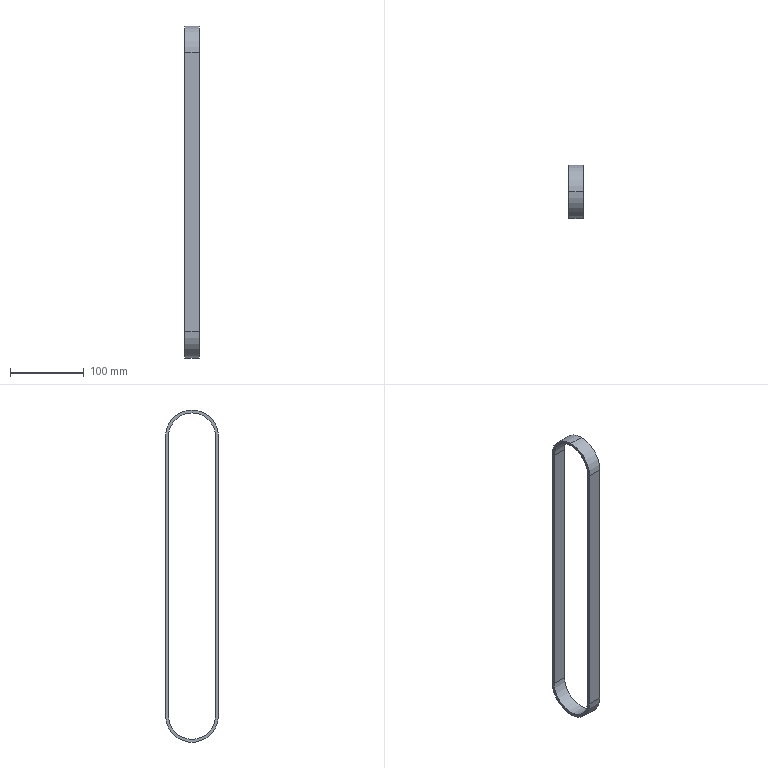Part | STEP file | PN_0034 (conveyor belt) | 1 solid | 12 faces | box 20 x 72 x 452 mm | volume 77890 mm3 | cylinder 6 | plane 6 | commonest cylinder face diameters 64 x3 72 x3
STEP:
#1=CARTESIAN_POINT('',(0.,0.,0.));
#2=DIRECTION('',(0.,0.,1.));
#3=DIRECTION('',(1.,0.,0.));
#4=AXIS2_PLACEMENT_3D('',#1,#2,#3);
#5=CARTESIAN_POINT('',(10.,32.,0.));
#6=VERTEX_POINT('',#5);
#7=CARTESIAN_POINT('',(-10.,32.,0.));
#8=VERTEX_POINT('',#7);
#9=CARTESIAN_POINT('',(10.,32.,0.));
#10=DIRECTION('',(-1.,0.,0.));
#11=VECTOR('',#10,1.);
#12=LINE('',#9,#11);
#13=CARTESIAN_POINT('',(10.,0.,0.));
#14=DIRECTION('',(-1.,0.,0.));
#15=DIRECTION('',(0.,0.,1.));
#16=AXIS2_PLACEMENT_3D('',#13,#14,#15);
#17=CYLINDRICAL_SURFACE('',#16,32.);
#18=CARTESIAN_POINT('',(1.571,0.));
#19=DIRECTION('',(0.,1.));
#20=VECTOR('',#19,1.);
#21=LINE('',#18,#20);
#22=(GEOMETRIC_REPRESENTATION_CONTEXT(2)PARAMETRIC_REPRESENTATION_CONTEXT()REPRESENTATION_CONTEXT('',''));
#23=DEFINITIONAL_REPRESENTATION('',(#21),#22);
#24=PCURVE('',#17,#23);
#25=CARTESIAN_POINT('',(10.,32.,0.));
#26=DIRECTION('',(0.,-1.,0.));
#27=DIRECTION('',(0.,0.,-1.));
#28=AXIS2_PLACEMENT_3D('',#25,#26,#27);
#29=PLANE('',#28);
#30=CARTESIAN_POINT('',(0.,0.));
#31=DIRECTION('',(0.,-1.));
#32=VECTOR('',#31,1.);
#33=LINE('',#30,#32);
#34=(GEOMETRIC_REPRESENTATION_CONTEXT(2)PARAMETRIC_REPRESENTATION_CONTEXT()REPRESENTATION_CONTEXT('',''));
#35=DEFINITIONAL_REPRESENTATION('',(#33),#34);
#36=PCURVE('',#29,#35);
#37=SURFACE_CURVE('',#12,(#24,#36),.PCURVE_S1.);
#38=EDGE_CURVE('',#6,#8,#37,.T.);
#39=ORIENTED_EDGE('',*,*,#38,.T.);
#40=CARTESIAN_POINT('',(-10.,0.,32.));
#41=VERTEX_POINT('',#40);
#42=CARTESIAN_POINT('',(-10.,0.,0.));
#43=DIRECTION('',(1.,0.,0.));
#44=DIRECTION('',(0.,0.,-1.));
#45=AXIS2_PLACEMENT_3D('',#42,#43,#44);
#46=CIRCLE('',#45,32.);
#47=CARTESIAN_POINT('',(3.142,20.));
#48=DIRECTION('',(-1.,0.));
#49=VECTOR('',#48,1.);
#50=LINE('',#47,#49);
#51=(GEOMETRIC_REPRESENTATION_CONTEXT(2)PARAMETRIC_REPRESENTATION_CONTEXT()REPRESENTATION_CONTEXT('',''));
#52=DEFINITIONAL_REPRESENTATION('',(#50),#51);
#53=PCURVE('',#17,#52);
#54=CARTESIAN_POINT('',(-10.,0.,0.));
#55=DIRECTION('',(1.,0.,0.));
#56=DIRECTION('',(0.,0.,-1.));
#57=AXIS2_PLACEMENT_3D('',#54,#55,#56);
#58=PLANE('',#57);
#59=CARTESIAN_POINT('',(0.,0.));
#60=DIRECTION('',(1.,0.));
#61=AXIS2_PLACEMENT_2D('',#59,#60);
#62=CIRCLE('',#61,32.);
#63=(GEOMETRIC_REPRESENTATION_CONTEXT(2)PARAMETRIC_REPRESENTATION_CONTEXT()REPRESENTATION_CONTEXT('',''));
#64=DEFINITIONAL_REPRESENTATION('',(#62),#63);
#65=PCURVE('',#58,#64);
#66=SURFACE_CURVE('',#46,(#53,#65),.PCURVE_S1.);
#67=EDGE_CURVE('',#8,#41,#66,.T.);
#68=ORIENTED_EDGE('',*,*,#67,.T.);
#69=CARTESIAN_POINT('',(10.,0.,32.));
#70=VERTEX_POINT('',#69);
#71=CARTESIAN_POINT('',(10.,0.,32.));
#72=DIRECTION('',(-1.,0.,0.));
#73=VECTOR('',#72,1.);
#74=LINE('',#71,#73);
#75=CARTESIAN_POINT('',(0.,0.));
#76=DIRECTION('',(0.,1.));
#77=VECTOR('',#76,1.);
#78=LINE('',#75,#77);
#79=(GEOMETRIC_REPRESENTATION_CONTEXT(2)PARAMETRIC_REPRESENTATION_CONTEXT()REPRESENTATION_CONTEXT('',''));
#80=DEFINITIONAL_REPRESENTATION('',(#78),#79);
#81=PCURVE('',#17,#80);
#82=CARTESIAN_POINT('',(10.,0.,0.));
#83=DIRECTION('',(-1.,0.,0.));
#84=DIRECTION('',(0.,0.,1.));
#85=AXIS2_PLACEMENT_3D('',#82,#83,#84);
#86=CYLINDRICAL_SURFACE('',#85,32.);
#87=CARTESIAN_POINT('',(6.283,0.));
#88=DIRECTION('',(0.,1.));
#89=VECTOR('',#88,1.);
#90=LINE('',#87,#89);
#91=(GEOMETRIC_REPRESENTATION_CONTEXT(2)PARAMETRIC_REPRESENTATION_CONTEXT()REPRESENTATION_CONTEXT('',''));
#92=DEFINITIONAL_REPRESENTATION('',(#90),#91);
#93=PCURVE('',#86,#92);
#94=SURFACE_CURVE('',#74,(#81,#93),.PCURVE_S1.);
#95=EDGE_CURVE('',#70,#41,#94,.T.);
#96=ORIENTED_EDGE('',*,*,#95,.F.);
#97=CARTESIAN_POINT('',(10.,0.,0.));
#98=DIRECTION('',(1.,0.,0.));
#99=DIRECTION('',(0.,0.,-1.));
#100=AXIS2_PLACEMENT_3D('',#97,#98,#99);
#101=CIRCLE('',#100,32.);
#102=CARTESIAN_POINT('',(3.142,0.));
#103=DIRECTION('',(-1.,0.));
#104=VECTOR('',#103,1.);
#105=LINE('',#102,#104);
#106=(GEOMETRIC_REPRESENTATION_CONTEXT(2)PARAMETRIC_REPRESENTATION_CONTEXT()REPRESENTATION_CONTEXT('',''));
#107=DEFINITIONAL_REPRESENTATION('',(#105),#106);
#108=PCURVE('',#17,#107);
#109=CARTESIAN_POINT('',(10.,0.,0.));
#110=DIRECTION('',(1.,0.,0.));
#111=DIRECTION('',(0.,0.,-1.));
#112=AXIS2_PLACEMENT_3D('',#109,#110,#111);
#113=PLANE('',#112);
#114=CARTESIAN_POINT('',(0.,0.));
#115=DIRECTION('',(1.,0.));
#116=AXIS2_PLACEMENT_2D('',#114,#115);
#117=CIRCLE('',#116,32.);
#118=(GEOMETRIC_REPRESENTATION_CONTEXT(2)PARAMETRIC_REPRESENTATION_CONTEXT()REPRESENTATION_CONTEXT('',''));
#119=DEFINITIONAL_REPRESENTATION('',(#117),#118);
#120=PCURVE('',#113,#119);
#121=SURFACE_CURVE('',#101,(#108,#120),.PCURVE_S1.);
#122=EDGE_CURVE('',#6,#70,#121,.T.);
#123=ORIENTED_EDGE('',*,*,#122,.F.);
#124=EDGE_LOOP('',(#39,#68,#96,#123));
#125=FACE_BOUND('',#124,.F.);
#126=ADVANCED_FACE('',(#125),#17,.F.);
#127=CARTESIAN_POINT('',(10.,0.,36.));
#128=VERTEX_POINT('',#127);
#129=CARTESIAN_POINT('',(10.,-36.,0.));
#130=VERTEX_POINT('',#129);
#131=CARTESIAN_POINT('',(10.,0.,0.));
#132=DIRECTION('',(1.,0.,0.));
#133=DIRECTION('',(0.,0.,-1.));
#134=AXIS2_PLACEMENT_3D('',#131,#132,#133);
#135=CIRCLE('',#134,36.);
#136=CARTESIAN_POINT('',(10.,0.,0.));
#137=DIRECTION('',(-1.,0.,0.));
#138=DIRECTION('',(0.,0.,1.));
#139=AXIS2_PLACEMENT_3D('',#136,#137,#138);
#140=CYLINDRICAL_SURFACE('',#139,36.);
#141=CARTESIAN_POINT('',(9.425,0.));
#142=DIRECTION('',(-1.,0.));
#143=VECTOR('',#142,1.);
#144=LINE('',#141,#143);
#145=(GEOMETRIC_REPRESENTATION_CONTEXT(2)PARAMETRIC_REPRESENTATION_CONTEXT()REPRESENTATION_CONTEXT('',''));
#146=DEFINITIONAL_REPRESENTATION('',(#144),#145);
#147=PCURVE('',#140,#146);
#148=CARTESIAN_POINT('',(0.,0.));
#149=DIRECTION('',(1.,0.));
#150=AXIS2_PLACEMENT_2D('',#148,#149);
#151=CIRCLE('',#150,36.);
#152=(GEOMETRIC_REPRESENTATION_CONTEXT(2)PARAMETRIC_REPRESENTATION_CONTEXT()REPRESENTATION_CONTEXT('',''));
#153=DEFINITIONAL_REPRESENTATION('',(#151),#152);
#154=PCURVE('',#113,#153);
#155=SURFACE_CURVE('',#135,(#147,#154),.PCURVE_S1.);
#156=EDGE_CURVE('',#128,#130,#155,.T.);
#157=ORIENTED_EDGE('',*,*,#156,.F.);
#158=CARTESIAN_POINT('',(-10.,0.,36.));
#159=VERTEX_POINT('',#158);
#160=CARTESIAN_POINT('',(10.,0.,36.));
#161=DIRECTION('',(-1.,0.,0.));
#162=VECTOR('',#161,1.);
#163=LINE('',#160,#162);
#164=CARTESIAN_POINT('',(6.283,0.));
#165=DIRECTION('',(0.,1.));
#166=VECTOR('',#165,1.);
#167=LINE('',#164,#166);
#168=(GEOMETRIC_REPRESENTATION_CONTEXT(2)PARAMETRIC_REPRESENTATION_CONTEXT()REPRESENTATION_CONTEXT('',''));
#169=DEFINITIONAL_REPRESENTATION('',(#167),#168);
#170=PCURVE('',#140,#169);
#171=CARTESIAN_POINT('',(10.,0.,0.));
#172=DIRECTION('',(-1.,0.,0.));
#173=DIRECTION('',(0.,0.,1.));
#174=AXIS2_PLACEMENT_3D('',#171,#172,#173);
#175=CYLINDRICAL_SURFACE('',#174,36.);
#176=CARTESIAN_POINT('',(0.,0.));
#177=DIRECTION('',(0.,1.));
#178=VECTOR('',#177,1.);
#179=LINE('',#176,#178);
#180=(GEOMETRIC_REPRESENTATION_CONTEXT(2)PARAMETRIC_REPRESENTATION_CONTEXT()REPRESENTATION_CONTEXT('',''));
#181=DEFINITIONAL_REPRESENTATION('',(#179),#180);
#182=PCURVE('',#175,#181);
#183=SURFACE_CURVE('',#163,(#170,#182),.PCURVE_S1.);
#184=EDGE_CURVE('',#128,#159,#183,.T.);
#185=ORIENTED_EDGE('',*,*,#184,.T.);
#186=CARTESIAN_POINT('',(-10.,-36.,0.));
#187=VERTEX_POINT('',#186);
#188=CARTESIAN_POINT('',(-10.,0.,0.));
#189=DIRECTION('',(1.,0.,0.));
#190=DIRECTION('',(0.,0.,-1.));
#191=AXIS2_PLACEMENT_3D('',#188,#189,#190);
#192=CIRCLE('',#191,36.);
#193=CARTESIAN_POINT('',(9.425,20.));
#194=DIRECTION('',(-1.,0.));
#195=VECTOR('',#194,1.);
#196=LINE('',#193,#195);
#197=(GEOMETRIC_REPRESENTATION_CONTEXT(2)PARAMETRIC_REPRESENTATION_CONTEXT()REPRESENTATION_CONTEXT('',''));
#198=DEFINITIONAL_REPRESENTATION('',(#196),#197);
#199=PCURVE('',#140,#198);
#200=CARTESIAN_POINT('',(0.,0.));
#201=DIRECTION('',(1.,0.));
#202=AXIS2_PLACEMENT_2D('',#200,#201);
#203=CIRCLE('',#202,36.);
#204=(GEOMETRIC_REPRESENTATION_CONTEXT(2)PARAMETRIC_REPRESENTATION_CONTEXT()REPRESENTATION_CONTEXT('',''));
#205=DEFINITIONAL_REPRESENTATION('',(#203),#204);
#206=PCURVE('',#58,#205);
#207=SURFACE_CURVE('',#192,(#199,#206),.PCURVE_S1.);
#208=EDGE_CURVE('',#159,#187,#207,.T.);
#209=ORIENTED_EDGE('',*,*,#208,.T.);
#210=CARTESIAN_POINT('',(10.,-36.,0.));
#211=DIRECTION('',(-1.,0.,0.));
#212=VECTOR('',#211,1.);
#213=LINE('',#210,#212);
#214=CARTESIAN_POINT('',(4.712,0.));
#215=DIRECTION('',(0.,1.));
#216=VECTOR('',#215,1.);
#217=LINE('',#214,#216);
#218=(GEOMETRIC_REPRESENTATION_CONTEXT(2)PARAMETRIC_REPRESENTATION_CONTEXT()REPRESENTATION_CONTEXT('',''));
#219=DEFINITIONAL_REPRESENTATION('',(#217),#218);
#220=PCURVE('',#140,#219);
#221=CARTESIAN_POINT('',(10.,-36.,0.));
#222=DIRECTION('',(0.,1.,0.));
#223=DIRECTION('',(0.,0.,1.));
#224=AXIS2_PLACEMENT_3D('',#221,#222,#223);
#225=PLANE('',#224);
#226=CARTESIAN_POINT('',(0.,0.));
#227=DIRECTION('',(0.,-1.));
#228=VECTOR('',#227,1.);
#229=LINE('',#226,#228);
#230=(GEOMETRIC_REPRESENTATION_CONTEXT(2)PARAMETRIC_REPRESENTATION_CONTEXT()REPRESENTATION_CONTEXT('',''));
#231=DEFINITIONAL_REPRESENTATION('',(#229),#230);
#232=PCURVE('',#225,#231);
#233=SURFACE_CURVE('',#213,(#220,#232),.PCURVE_S1.);
#234=EDGE_CURVE('',#130,#187,#233,.T.);
#235=ORIENTED_EDGE('',*,*,#234,.F.);
#236=EDGE_LOOP('',(#157,#185,#209,#235));
#237=FACE_BOUND('',#236,.T.);
#238=ADVANCED_FACE('',(#237),#140,.T.);
#239=CARTESIAN_POINT('',(10.,36.,0.));
#240=VERTEX_POINT('',#239);
#241=CARTESIAN_POINT('',(10.,0.,0.));
#242=DIRECTION('',(1.,0.,0.));
#243=DIRECTION('',(0.,0.,-1.));
#244=AXIS2_PLACEMENT_3D('',#241,#242,#243);
#245=CIRCLE('',#244,36.);
#246=CARTESIAN_POINT('',(0.,0.));
#247=DIRECTION('',(1.,0.));
#248=AXIS2_PLACEMENT_2D('',#246,#247);
#249=CIRCLE('',#248,36.);
#250=(GEOMETRIC_REPRESENTATION_CONTEXT(2)PARAMETRIC_REPRESENTATION_CONTEXT()REPRESENTATION_CONTEXT('',''));
#251=DEFINITIONAL_REPRESENTATION('',(#249),#250);
#252=PCURVE('',#113,#251);
#253=CARTESIAN_POINT('',(3.142,0.));
#254=DIRECTION('',(-1.,0.));
#255=VECTOR('',#254,1.);
#256=LINE('',#253,#255);
#257=(GEOMETRIC_REPRESENTATION_CONTEXT(2)PARAMETRIC_REPRESENTATION_CONTEXT()REPRESENTATION_CONTEXT('',''));
#258=DEFINITIONAL_REPRESENTATION('',(#256),#257);
#259=PCURVE('',#175,#258);
#260=SURFACE_CURVE('',#245,(#252,#259),.PCURVE_S1.);
#261=EDGE_CURVE('',#240,#128,#260,.T.);
#262=ORIENTED_EDGE('',*,*,#261,.T.);
#263=ORIENTED_EDGE('',*,*,#156,.T.);
#264=CARTESIAN_POINT('',(10.,-36.,-380.));
#265=VERTEX_POINT('',#264);
#266=CARTESIAN_POINT('',(10.,-36.,0.));
#267=DIRECTION('',(0.,0.,-1.));
#268=VECTOR('',#267,1.);
#269=LINE('',#266,#268);
#270=CARTESIAN_POINT('',(0.,-36.));
#271=DIRECTION('',(1.,0.));
#272=VECTOR('',#271,1.);
#273=LINE('',#270,#272);
#274=(GEOMETRIC_REPRESENTATION_CONTEXT(2)PARAMETRIC_REPRESENTATION_CONTEXT()REPRESENTATION_CONTEXT('',''));
#275=DEFINITIONAL_REPRESENTATION('',(#273),#274);
#276=PCURVE('',#113,#275);
#277=CARTESIAN_POINT('',(0.,0.));
#278=DIRECTION('',(-1.,0.));
#279=VECTOR('',#278,1.);
#280=LINE('',#277,#279);
#281=(GEOMETRIC_REPRESENTATION_CONTEXT(2)PARAMETRIC_REPRESENTATION_CONTEXT()REPRESENTATION_CONTEXT('',''));
#282=DEFINITIONAL_REPRESENTATION('',(#280),#281);
#283=PCURVE('',#225,#282);
#284=SURFACE_CURVE('',#269,(#276,#283),.PCURVE_S1.);
#285=EDGE_CURVE('',#130,#265,#284,.T.);
#286=ORIENTED_EDGE('',*,*,#285,.T.);
#287=CARTESIAN_POINT('',(10.,36.,-380.));
#288=VERTEX_POINT('',#287);
#289=CARTESIAN_POINT('',(10.,0.,-380.));
#290=DIRECTION('',(1.,0.,0.));
#291=DIRECTION('',(0.,0.,-1.));
#292=AXIS2_PLACEMENT_3D('',#289,#290,#291);
#293=CIRCLE('',#292,36.);
#294=CARTESIAN_POINT('',(380.,0.));
#295=DIRECTION('',(1.,0.));
#296=AXIS2_PLACEMENT_2D('',#294,#295);
#297=CIRCLE('',#296,36.);
#298=(GEOMETRIC_REPRESENTATION_CONTEXT(2)PARAMETRIC_REPRESENTATION_CONTEXT()REPRESENTATION_CONTEXT('',''));
#299=DEFINITIONAL_REPRESENTATION('',(#297),#298);
#300=PCURVE('',#113,#299);
#301=CARTESIAN_POINT('',(10.,0.,-380.));
#302=DIRECTION('',(-1.,0.,0.));
#303=DIRECTION('',(0.,0.,1.));
#304=AXIS2_PLACEMENT_3D('',#301,#302,#303);
#305=CYLINDRICAL_SURFACE('',#304,36.);
#306=CARTESIAN_POINT('',(9.425,0.));
#307=DIRECTION('',(-1.,0.));
#308=VECTOR('',#307,1.);
#309=LINE('',#306,#308);
#310=(GEOMETRIC_REPRESENTATION_CONTEXT(2)PARAMETRIC_REPRESENTATION_CONTEXT()REPRESENTATION_CONTEXT('',''));
#311=DEFINITIONAL_REPRESENTATION('',(#309),#310);
#312=PCURVE('',#305,#311);
#313=SURFACE_CURVE('',#293,(#300,#312),.PCURVE_S1.);
#314=EDGE_CURVE('',#265,#288,#313,.T.);
#315=ORIENTED_EDGE('',*,*,#314,.T.);
#316=CARTESIAN_POINT('',(10.,36.,0.));
#317=DIRECTION('',(0.,0.,1.));
#318=VECTOR('',#317,1.);
#319=LINE('',#316,#318);
#320=CARTESIAN_POINT('',(0.,36.));
#321=DIRECTION('',(-1.,0.));
#322=VECTOR('',#321,1.);
#323=LINE('',#320,#322);
#324=(GEOMETRIC_REPRESENTATION_CONTEXT(2)PARAMETRIC_REPRESENTATION_CONTEXT()REPRESENTATION_CONTEXT('',''));
#325=DEFINITIONAL_REPRESENTATION('',(#323),#324);
#326=PCURVE('',#113,#325);
#327=CARTESIAN_POINT('',(10.,36.,0.));
#328=DIRECTION('',(0.,-1.,0.));
#329=DIRECTION('',(0.,0.,-1.));
#330=AXIS2_PLACEMENT_3D('',#327,#328,#329);
#331=PLANE('',#330);
#332=CARTESIAN_POINT('',(0.,0.));
#333=DIRECTION('',(-1.,0.));
#334=VECTOR('',#333,1.);
#335=LINE('',#332,#334);
#336=(GEOMETRIC_REPRESENTATION_CONTEXT(2)PARAMETRIC_REPRESENTATION_CONTEXT()REPRESENTATION_CONTEXT('',''));
#337=DEFINITIONAL_REPRESENTATION('',(#335),#336);
#338=PCURVE('',#331,#337);
#339=SURFACE_CURVE('',#319,(#326,#338),.PCURVE_S1.);
#340=EDGE_CURVE('',#288,#240,#339,.T.);
#341=ORIENTED_EDGE('',*,*,#340,.T.);
#342=EDGE_LOOP('',(#262,#263,#286,#315,#341));
#343=FACE_BOUND('',#342,.T.);
#344=CARTESIAN_POINT('',(10.,-32.,0.));
#345=VERTEX_POINT('',#344);
#346=CARTESIAN_POINT('',(10.,-32.,-380.));
#347=VERTEX_POINT('',#346);
#348=CARTESIAN_POINT('',(10.,-32.,0.));
#349=DIRECTION('',(0.,0.,-1.));
#350=VECTOR('',#349,1.);
#351=LINE('',#348,#350);
#352=CARTESIAN_POINT('',(0.,-32.));
#353=DIRECTION('',(1.,0.));
#354=VECTOR('',#353,1.);
#355=LINE('',#352,#354);
#356=(GEOMETRIC_REPRESENTATION_CONTEXT(2)PARAMETRIC_REPRESENTATION_CONTEXT()REPRESENTATION_CONTEXT('',''));
#357=DEFINITIONAL_REPRESENTATION('',(#355),#356);
#358=PCURVE('',#113,#357);
#359=CARTESIAN_POINT('',(10.,-32.,0.));
#360=DIRECTION('',(0.,1.,0.));
#361=DIRECTION('',(0.,0.,1.));
#362=AXIS2_PLACEMENT_3D('',#359,#360,#361);
#363=PLANE('',#362);
#364=CARTESIAN_POINT('',(0.,0.));
#365=DIRECTION('',(-1.,0.));
#366=VECTOR('',#365,1.);
#367=LINE('',#364,#366);
#368=(GEOMETRIC_REPRESENTATION_CONTEXT(2)PARAMETRIC_REPRESENTATION_CONTEXT()REPRESENTATION_CONTEXT('',''));
#369=DEFINITIONAL_REPRESENTATION('',(#367),#368);
#370=PCURVE('',#363,#369);
#371=SURFACE_CURVE('',#351,(#358,#370),.PCURVE_S1.);
#372=EDGE_CURVE('',#345,#347,#371,.T.);
#373=ORIENTED_EDGE('',*,*,#372,.F.);
#374=CARTESIAN_POINT('',(10.,0.,0.));
#375=DIRECTION('',(1.,0.,0.));
#376=DIRECTION('',(0.,0.,-1.));
#377=AXIS2_PLACEMENT_3D('',#374,#375,#376);
#378=CIRCLE('',#377,32.);
#379=CARTESIAN_POINT('',(0.,0.));
#380=DIRECTION('',(1.,0.));
#381=AXIS2_PLACEMENT_2D('',#379,#380);
#382=CIRCLE('',#381,32.);
#383=(GEOMETRIC_REPRESENTATION_CONTEXT(2)PARAMETRIC_REPRESENTATION_CONTEXT()REPRESENTATION_CONTEXT('',''));
#384=DEFINITIONAL_REPRESENTATION('',(#382),#383);
#385=PCURVE('',#113,#384);
#386=CARTESIAN_POINT('',(9.425,0.));
#387=DIRECTION('',(-1.,0.));
#388=VECTOR('',#387,1.);
#389=LINE('',#386,#388);
#390=(GEOMETRIC_REPRESENTATION_CONTEXT(2)PARAMETRIC_REPRESENTATION_CONTEXT()REPRESENTATION_CONTEXT('',''));
#391=DEFINITIONAL_REPRESENTATION('',(#389),#390);
#392=PCURVE('',#86,#391);
#393=SURFACE_CURVE('',#378,(#385,#392),.PCURVE_S1.);
#394=EDGE_CURVE('',#70,#345,#393,.T.);
#395=ORIENTED_EDGE('',*,*,#394,.F.);
#396=ORIENTED_EDGE('',*,*,#122,.F.);
#397=CARTESIAN_POINT('',(10.,32.,-380.));
#398=VERTEX_POINT('',#397);
#399=CARTESIAN_POINT('',(10.,32.,0.));
#400=DIRECTION('',(0.,0.,1.));
#401=VECTOR('',#400,1.);
#402=LINE('',#399,#401);
#403=CARTESIAN_POINT('',(0.,32.));
#404=DIRECTION('',(-1.,0.));
#405=VECTOR('',#404,1.);
#406=LINE('',#403,#405);
#407=(GEOMETRIC_REPRESENTATION_CONTEXT(2)PARAMETRIC_REPRESENTATION_CONTEXT()REPRESENTATION_CONTEXT('',''));
#408=DEFINITIONAL_REPRESENTATION('',(#406),#407);
#409=PCURVE('',#113,#408);
#410=CARTESIAN_POINT('',(0.,0.));
#411=DIRECTION('',(-1.,0.));
#412=VECTOR('',#411,1.);
#413=LINE('',#410,#412);
#414=(GEOMETRIC_REPRESENTATION_CONTEXT(2)PARAMETRIC_REPRESENTATION_CONTEXT()REPRESENTATION_CONTEXT('',''));
#415=DEFINITIONAL_REPRESENTATION('',(#413),#414);
#416=PCURVE('',#29,#415);
#417=SURFACE_CURVE('',#402,(#409,#416),.PCURVE_S1.);
#418=EDGE_CURVE('',#398,#6,#417,.T.);
#419=ORIENTED_EDGE('',*,*,#418,.F.);
#420=CARTESIAN_POINT('',(10.,0.,-380.));
#421=DIRECTION('',(1.,0.,0.));
#422=DIRECTION('',(0.,0.,-1.));
#423=AXIS2_PLACEMENT_3D('',#420,#421,#422);
#424=CIRCLE('',#423,32.);
#425=CARTESIAN_POINT('',(380.,0.));
#426=DIRECTION('',(1.,0.));
#427=AXIS2_PLACEMENT_2D('',#425,#426);
#428=CIRCLE('',#427,32.);
#429=(GEOMETRIC_REPRESENTATION_CONTEXT(2)PARAMETRIC_REPRESENTATION_CONTEXT()REPRESENTATION_CONTEXT('',''));
#430=DEFINITIONAL_REPRESENTATION('',(#428),#429);
#431=PCURVE('',#113,#430);
#432=CARTESIAN_POINT('',(10.,0.,-380.));
#433=DIRECTION('',(-1.,0.,0.));
#434=DIRECTION('',(0.,0.,1.));
#435=AXIS2_PLACEMENT_3D('',#432,#433,#434);
#436=CYLINDRICAL_SURFACE('',#435,32.);
#437=CARTESIAN_POINT('',(9.425,0.));
#438=DIRECTION('',(-1.,0.));
#439=VECTOR('',#438,1.);
#440=LINE('',#437,#439);
#441=(GEOMETRIC_REPRESENTATION_CONTEXT(2)PARAMETRIC_REPRESENTATION_CONTEXT()REPRESENTATION_CONTEXT('',''));
#442=DEFINITIONAL_REPRESENTATION('',(#440),#441);
#443=PCURVE('',#436,#442);
#444=SURFACE_CURVE('',#424,(#431,#443),.PCURVE_S1.);
#445=EDGE_CURVE('',#347,#398,#444,.T.);
#446=ORIENTED_EDGE('',*,*,#445,.F.);
#447=EDGE_LOOP('',(#373,#395,#396,#419,#446));
#448=FACE_BOUND('',#447,.T.);
#449=ADVANCED_FACE('',(#343,#448),#113,.T.);
#450=CARTESIAN_POINT('',(-10.,36.,0.));
#451=VERTEX_POINT('',#450);
#452=CARTESIAN_POINT('',(-10.,0.,0.));
#453=DIRECTION('',(1.,0.,0.));
#454=DIRECTION('',(0.,0.,-1.));
#455=AXIS2_PLACEMENT_3D('',#452,#453,#454);
#456=CIRCLE('',#455,36.);
#457=CARTESIAN_POINT('',(0.,0.));
#458=DIRECTION('',(1.,0.));
#459=AXIS2_PLACEMENT_2D('',#457,#458);
#460=CIRCLE('',#459,36.);
#461=(GEOMETRIC_REPRESENTATION_CONTEXT(2)PARAMETRIC_REPRESENTATION_CONTEXT()REPRESENTATION_CONTEXT('',''));
#462=DEFINITIONAL_REPRESENTATION('',(#460),#461);
#463=PCURVE('',#58,#462);
#464=CARTESIAN_POINT('',(3.142,20.));
#465=DIRECTION('',(-1.,0.));
#466=VECTOR('',#465,1.);
#467=LINE('',#464,#466);
#468=(GEOMETRIC_REPRESENTATION_CONTEXT(2)PARAMETRIC_REPRESENTATION_CONTEXT()REPRESENTATION_CONTEXT('',''));
#469=DEFINITIONAL_REPRESENTATION('',(#467),#468);
#470=PCURVE('',#175,#469);
#471=SURFACE_CURVE('',#456,(#463,#470),.PCURVE_S1.);
#472=EDGE_CURVE('',#451,#159,#471,.T.);
#473=ORIENTED_EDGE('',*,*,#472,.F.);
#474=CARTESIAN_POINT('',(-10.,36.,-380.));
#475=VERTEX_POINT('',#474);
#476=CARTESIAN_POINT('',(-10.,36.,0.));
#477=DIRECTION('',(0.,0.,1.));
#478=VECTOR('',#477,1.);
#479=LINE('',#476,#478);
#480=CARTESIAN_POINT('',(0.,36.));
#481=DIRECTION('',(-1.,0.));
#482=VECTOR('',#481,1.);
#483=LINE('',#480,#482);
#484=(GEOMETRIC_REPRESENTATION_CONTEXT(2)PARAMETRIC_REPRESENTATION_CONTEXT()REPRESENTATION_CONTEXT('',''));
#485=DEFINITIONAL_REPRESENTATION('',(#483),#484);
#486=PCURVE('',#58,#485);
#487=CARTESIAN_POINT('',(0.,-20.));
#488=DIRECTION('',(-1.,0.));
#489=VECTOR('',#488,1.);
#490=LINE('',#487,#489);
#491=(GEOMETRIC_REPRESENTATION_CONTEXT(2)PARAMETRIC_REPRESENTATION_CONTEXT()REPRESENTATION_CONTEXT('',''));
#492=DEFINITIONAL_REPRESENTATION('',(#490),#491);
#493=PCURVE('',#331,#492);
#494=SURFACE_CURVE('',#479,(#486,#493),.PCURVE_S1.);
#495=EDGE_CURVE('',#475,#451,#494,.T.);
#496=ORIENTED_EDGE('',*,*,#495,.F.);
#497=CARTESIAN_POINT('',(-10.,-36.,-380.));
#498=VERTEX_POINT('',#497);
#499=CARTESIAN_POINT('',(-10.,0.,-380.));
#500=DIRECTION('',(1.,0.,0.));
#501=DIRECTION('',(0.,0.,-1.));
#502=AXIS2_PLACEMENT_3D('',#499,#500,#501);
#503=CIRCLE('',#502,36.);
#504=CARTESIAN_POINT('',(380.,0.));
#505=DIRECTION('',(1.,0.));
#506=AXIS2_PLACEMENT_2D('',#504,#505);
#507=CIRCLE('',#506,36.);
#508=(GEOMETRIC_REPRESENTATION_CONTEXT(2)PARAMETRIC_REPRESENTATION_CONTEXT()REPRESENTATION_CONTEXT('',''));
#509=DEFINITIONAL_REPRESENTATION('',(#507),#508);
#510=PCURVE('',#58,#509);
#511=CARTESIAN_POINT('',(9.425,20.));
#512=DIRECTION('',(-1.,0.));
#513=VECTOR('',#512,1.);
#514=LINE('',#511,#513);
#515=(GEOMETRIC_REPRESENTATION_CONTEXT(2)PARAMETRIC_REPRESENTATION_CONTEXT()REPRESENTATION_CONTEXT('',''));
#516=DEFINITIONAL_REPRESENTATION('',(#514),#515);
#517=PCURVE('',#305,#516);
#518=SURFACE_CURVE('',#503,(#510,#517),.PCURVE_S1.);
#519=EDGE_CURVE('',#498,#475,#518,.T.);
#520=ORIENTED_EDGE('',*,*,#519,.F.);
#521=CARTESIAN_POINT('',(-10.,-36.,0.));
#522=DIRECTION('',(0.,0.,-1.));
#523=VECTOR('',#522,1.);
#524=LINE('',#521,#523);
#525=CARTESIAN_POINT('',(0.,-36.));
#526=DIRECTION('',(1.,0.));
#527=VECTOR('',#526,1.);
#528=LINE('',#525,#527);
#529=(GEOMETRIC_REPRESENTATION_CONTEXT(2)PARAMETRIC_REPRESENTATION_CONTEXT()REPRESENTATION_CONTEXT('',''));
#530=DEFINITIONAL_REPRESENTATION('',(#528),#529);
#531=PCURVE('',#58,#530);
#532=CARTESIAN_POINT('',(0.,-20.));
#533=DIRECTION('',(-1.,0.));
#534=VECTOR('',#533,1.);
#535=LINE('',#532,#534);
#536=(GEOMETRIC_REPRESENTATION_CONTEXT(2)PARAMETRIC_REPRESENTATION_CONTEXT()REPRESENTATION_CONTEXT('',''));
#537=DEFINITIONAL_REPRESENTATION('',(#535),#536);
#538=PCURVE('',#225,#537);
#539=SURFACE_CURVE('',#524,(#531,#538),.PCURVE_S1.);
#540=EDGE_CURVE('',#187,#498,#539,.T.);
#541=ORIENTED_EDGE('',*,*,#540,.F.);
#542=ORIENTED_EDGE('',*,*,#208,.F.);
#543=EDGE_LOOP('',(#473,#496,#520,#541,#542));
#544=FACE_BOUND('',#543,.T.);
#545=ORIENTED_EDGE('',*,*,#67,.T.);
#546=CARTESIAN_POINT('',(-10.,-32.,0.));
#547=VERTEX_POINT('',#546);
#548=CARTESIAN_POINT('',(-10.,0.,0.));
#549=DIRECTION('',(1.,0.,0.));
#550=DIRECTION('',(0.,0.,-1.));
#551=AXIS2_PLACEMENT_3D('',#548,#549,#550);
#552=CIRCLE('',#551,32.);
#553=CARTESIAN_POINT('',(0.,0.));
#554=DIRECTION('',(1.,0.));
#555=AXIS2_PLACEMENT_2D('',#553,#554);
#556=CIRCLE('',#555,32.);
#557=(GEOMETRIC_REPRESENTATION_CONTEXT(2)PARAMETRIC_REPRESENTATION_CONTEXT()REPRESENTATION_CONTEXT('',''));
#558=DEFINITIONAL_REPRESENTATION('',(#556),#557);
#559=PCURVE('',#58,#558);
#560=CARTESIAN_POINT('',(9.425,20.));
#561=DIRECTION('',(-1.,0.));
#562=VECTOR('',#561,1.);
#563=LINE('',#560,#562);
#564=(GEOMETRIC_REPRESENTATION_CONTEXT(2)PARAMETRIC_REPRESENTATION_CONTEXT()REPRESENTATION_CONTEXT('',''));
#565=DEFINITIONAL_REPRESENTATION('',(#563),#564);
#566=PCURVE('',#86,#565);
#567=SURFACE_CURVE('',#552,(#559,#566),.PCURVE_S1.);
#568=EDGE_CURVE('',#41,#547,#567,.T.);
#569=ORIENTED_EDGE('',*,*,#568,.T.);
#570=CARTESIAN_POINT('',(-10.,-32.,-380.));
#571=VERTEX_POINT('',#570);
#572=CARTESIAN_POINT('',(-10.,-32.,0.));
#573=DIRECTION('',(0.,0.,-1.));
#574=VECTOR('',#573,1.);
#575=LINE('',#572,#574);
#576=CARTESIAN_POINT('',(0.,-32.));
#577=DIRECTION('',(1.,0.));
#578=VECTOR('',#577,1.);
#579=LINE('',#576,#578);
#580=(GEOMETRIC_REPRESENTATION_CONTEXT(2)PARAMETRIC_REPRESENTATION_CONTEXT()REPRESENTATION_CONTEXT('',''));
#581=DEFINITIONAL_REPRESENTATION('',(#579),#580);
#582=PCURVE('',#58,#581);
#583=CARTESIAN_POINT('',(0.,-20.));
#584=DIRECTION('',(-1.,0.));
#585=VECTOR('',#584,1.);
#586=LINE('',#583,#585);
#587=(GEOMETRIC_REPRESENTATION_CONTEXT(2)PARAMETRIC_REPRESENTATION_CONTEXT()REPRESENTATION_CONTEXT('',''));
#588=DEFINITIONAL_REPRESENTATION('',(#586),#587);
#589=PCURVE('',#363,#588);
#590=SURFACE_CURVE('',#575,(#582,#589),.PCURVE_S1.);
#591=EDGE_CURVE('',#547,#571,#590,.T.);
#592=ORIENTED_EDGE('',*,*,#591,.T.);
#593=CARTESIAN_POINT('',(-10.,32.,-380.));
#594=VERTEX_POINT('',#593);
#595=CARTESIAN_POINT('',(-10.,0.,-380.));
#596=DIRECTION('',(1.,0.,0.));
#597=DIRECTION('',(0.,0.,-1.));
#598=AXIS2_PLACEMENT_3D('',#595,#596,#597);
#599=CIRCLE('',#598,32.);
#600=CARTESIAN_POINT('',(380.,0.));
#601=DIRECTION('',(1.,0.));
#602=AXIS2_PLACEMENT_2D('',#600,#601);
#603=CIRCLE('',#602,32.);
#604=(GEOMETRIC_REPRESENTATION_CONTEXT(2)PARAMETRIC_REPRESENTATION_CONTEXT()REPRESENTATION_CONTEXT('',''));
#605=DEFINITIONAL_REPRESENTATION('',(#603),#604);
#606=PCURVE('',#58,#605);
#607=CARTESIAN_POINT('',(9.425,20.));
#608=DIRECTION('',(-1.,0.));
#609=VECTOR('',#608,1.);
#610=LINE('',#607,#609);
#611=(GEOMETRIC_REPRESENTATION_CONTEXT(2)PARAMETRIC_REPRESENTATION_CONTEXT()REPRESENTATION_CONTEXT('',''));
#612=DEFINITIONAL_REPRESENTATION('',(#610),#611);
#613=PCURVE('',#436,#612);
#614=SURFACE_CURVE('',#599,(#606,#613),.PCURVE_S1.);
#615=EDGE_CURVE('',#571,#594,#614,.T.);
#616=ORIENTED_EDGE('',*,*,#615,.T.);
#617=CARTESIAN_POINT('',(-10.,32.,0.));
#618=DIRECTION('',(0.,0.,1.));
#619=VECTOR('',#618,1.);
#620=LINE('',#617,#619);
#621=CARTESIAN_POINT('',(0.,32.));
#622=DIRECTION('',(-1.,0.));
#623=VECTOR('',#622,1.);
#624=LINE('',#621,#623);
#625=(GEOMETRIC_REPRESENTATION_CONTEXT(2)PARAMETRIC_REPRESENTATION_CONTEXT()REPRESENTATION_CONTEXT('',''));
#626=DEFINITIONAL_REPRESENTATION('',(#624),#625);
#627=PCURVE('',#58,#626);
#628=CARTESIAN_POINT('',(0.,-20.));
#629=DIRECTION('',(-1.,0.));
#630=VECTOR('',#629,1.);
#631=LINE('',#628,#630);
#632=(GEOMETRIC_REPRESENTATION_CONTEXT(2)PARAMETRIC_REPRESENTATION_CONTEXT()REPRESENTATION_CONTEXT('',''));
#633=DEFINITIONAL_REPRESENTATION('',(#631),#632);
#634=PCURVE('',#29,#633);
#635=SURFACE_CURVE('',#620,(#627,#634),.PCURVE_S1.);
#636=EDGE_CURVE('',#594,#8,#635,.T.);
#637=ORIENTED_EDGE('',*,*,#636,.T.);
#638=EDGE_LOOP('',(#545,#569,#592,#616,#637));
#639=FACE_BOUND('',#638,.T.);
#640=ADVANCED_FACE('',(#544,#639),#58,.F.);
#641=ORIENTED_EDGE('',*,*,#184,.F.);
#642=ORIENTED_EDGE('',*,*,#261,.F.);
#643=CARTESIAN_POINT('',(10.,36.,0.));
#644=DIRECTION('',(-1.,0.,0.));
#645=VECTOR('',#644,1.);
#646=LINE('',#643,#645);
#647=CARTESIAN_POINT('',(1.571,0.));
#648=DIRECTION('',(0.,1.));
#649=VECTOR('',#648,1.);
#650=LINE('',#647,#649);
#651=(GEOMETRIC_REPRESENTATION_CONTEXT(2)PARAMETRIC_REPRESENTATION_CONTEXT()REPRESENTATION_CONTEXT('',''));
#652=DEFINITIONAL_REPRESENTATION('',(#650),#651);
#653=PCURVE('',#175,#652);
#654=CARTESIAN_POINT('',(0.,0.));
#655=DIRECTION('',(0.,-1.));
#656=VECTOR('',#655,1.);
#657=LINE('',#654,#656);
#658=(GEOMETRIC_REPRESENTATION_CONTEXT(2)PARAMETRIC_REPRESENTATION_CONTEXT()REPRESENTATION_CONTEXT('',''));
#659=DEFINITIONAL_REPRESENTATION('',(#657),#658);
#660=PCURVE('',#331,#659);
#661=SURFACE_CURVE('',#646,(#653,#660),.PCURVE_S1.);
#662=EDGE_CURVE('',#240,#451,#661,.T.);
#663=ORIENTED_EDGE('',*,*,#662,.T.);
#664=ORIENTED_EDGE('',*,*,#472,.T.);
#665=EDGE_LOOP('',(#641,#642,#663,#664));
#666=FACE_BOUND('',#665,.T.);
#667=ADVANCED_FACE('',(#666),#175,.T.);
#668=ORIENTED_EDGE('',*,*,#540,.T.);
#669=CARTESIAN_POINT('',(10.,-36.,-380.));
#670=DIRECTION('',(-1.,0.,0.));
#671=VECTOR('',#670,1.);
#672=LINE('',#669,#671);
#673=CARTESIAN_POINT('',(-380.,0.));
#674=DIRECTION('',(0.,-1.));
#675=VECTOR('',#674,1.);
#676=LINE('',#673,#675);
#677=(GEOMETRIC_REPRESENTATION_CONTEXT(2)PARAMETRIC_REPRESENTATION_CONTEXT()REPRESENTATION_CONTEXT('',''));
#678=DEFINITIONAL_REPRESENTATION('',(#676),#677);
#679=PCURVE('',#225,#678);
#680=CARTESIAN_POINT('',(4.712,0.));
#681=DIRECTION('',(0.,1.));
#682=VECTOR('',#681,1.);
#683=LINE('',#680,#682);
#684=(GEOMETRIC_REPRESENTATION_CONTEXT(2)PARAMETRIC_REPRESENTATION_CONTEXT()REPRESENTATION_CONTEXT('',''));
#685=DEFINITIONAL_REPRESENTATION('',(#683),#684);
#686=PCURVE('',#305,#685);
#687=SURFACE_CURVE('',#672,(#679,#686),.PCURVE_S1.);
#688=EDGE_CURVE('',#265,#498,#687,.T.);
#689=ORIENTED_EDGE('',*,*,#688,.F.);
#690=ORIENTED_EDGE('',*,*,#285,.F.);
#691=ORIENTED_EDGE('',*,*,#234,.T.);
#692=EDGE_LOOP('',(#668,#689,#690,#691));
#693=FACE_BOUND('',#692,.T.);
#694=ADVANCED_FACE('',(#693),#225,.F.);
#695=ORIENTED_EDGE('',*,*,#519,.T.);
#696=CARTESIAN_POINT('',(10.,36.,-380.));
#697=DIRECTION('',(-1.,0.,0.));
#698=VECTOR('',#697,1.);
#699=LINE('',#696,#698);
#700=CARTESIAN_POINT('',(1.571,0.));
#701=DIRECTION('',(0.,1.));
#702=VECTOR('',#701,1.);
#703=LINE('',#700,#702);
#704=(GEOMETRIC_REPRESENTATION_CONTEXT(2)PARAMETRIC_REPRESENTATION_CONTEXT()REPRESENTATION_CONTEXT('',''));
#705=DEFINITIONAL_REPRESENTATION('',(#703),#704);
#706=PCURVE('',#305,#705);
#707=CARTESIAN_POINT('',(380.,0.));
#708=DIRECTION('',(0.,-1.));
#709=VECTOR('',#708,1.);
#710=LINE('',#707,#709);
#711=(GEOMETRIC_REPRESENTATION_CONTEXT(2)PARAMETRIC_REPRESENTATION_CONTEXT()REPRESENTATION_CONTEXT('',''));
#712=DEFINITIONAL_REPRESENTATION('',(#710),#711);
#713=PCURVE('',#331,#712);
#714=SURFACE_CURVE('',#699,(#706,#713),.PCURVE_S1.);
#715=EDGE_CURVE('',#288,#475,#714,.T.);
#716=ORIENTED_EDGE('',*,*,#715,.F.);
#717=ORIENTED_EDGE('',*,*,#314,.F.);
#718=ORIENTED_EDGE('',*,*,#688,.T.);
#719=EDGE_LOOP('',(#695,#716,#717,#718));
#720=FACE_BOUND('',#719,.T.);
#721=ADVANCED_FACE('',(#720),#305,.T.);
#722=ORIENTED_EDGE('',*,*,#495,.T.);
#723=ORIENTED_EDGE('',*,*,#662,.F.);
#724=ORIENTED_EDGE('',*,*,#340,.F.);
#725=ORIENTED_EDGE('',*,*,#715,.T.);
#726=EDGE_LOOP('',(#722,#723,#724,#725));
#727=FACE_BOUND('',#726,.T.);
#728=ADVANCED_FACE('',(#727),#331,.F.);
#729=ORIENTED_EDGE('',*,*,#568,.T.);
#730=CARTESIAN_POINT('',(10.,-32.,0.));
#731=DIRECTION('',(-1.,0.,0.));
#732=VECTOR('',#731,1.);
#733=LINE('',#730,#732);
#734=CARTESIAN_POINT('',(4.712,0.));
#735=DIRECTION('',(0.,1.));
#736=VECTOR('',#735,1.);
#737=LINE('',#734,#736);
#738=(GEOMETRIC_REPRESENTATION_CONTEXT(2)PARAMETRIC_REPRESENTATION_CONTEXT()REPRESENTATION_CONTEXT('',''));
#739=DEFINITIONAL_REPRESENTATION('',(#737),#738);
#740=PCURVE('',#86,#739);
#741=CARTESIAN_POINT('',(0.,0.));
#742=DIRECTION('',(0.,-1.));
#743=VECTOR('',#742,1.);
#744=LINE('',#741,#743);
#745=(GEOMETRIC_REPRESENTATION_CONTEXT(2)PARAMETRIC_REPRESENTATION_CONTEXT()REPRESENTATION_CONTEXT('',''));
#746=DEFINITIONAL_REPRESENTATION('',(#744),#745);
#747=PCURVE('',#363,#746);
#748=SURFACE_CURVE('',#733,(#740,#747),.PCURVE_S1.);
#749=EDGE_CURVE('',#345,#547,#748,.T.);
#750=ORIENTED_EDGE('',*,*,#749,.F.);
#751=ORIENTED_EDGE('',*,*,#394,.F.);
#752=ORIENTED_EDGE('',*,*,#95,.T.);
#753=EDGE_LOOP('',(#729,#750,#751,#752));
#754=FACE_BOUND('',#753,.F.);
#755=ADVANCED_FACE('',(#754),#86,.F.);
#756=ORIENTED_EDGE('',*,*,#591,.F.);
#757=ORIENTED_EDGE('',*,*,#749,.F.);
#758=ORIENTED_EDGE('',*,*,#372,.T.);
#759=CARTESIAN_POINT('',(10.,-32.,-380.));
#760=DIRECTION('',(-1.,0.,0.));
#761=VECTOR('',#760,1.);
#762=LINE('',#759,#761);
#763=CARTESIAN_POINT('',(-380.,0.));
#764=DIRECTION('',(0.,-1.));
#765=VECTOR('',#764,1.);
#766=LINE('',#763,#765);
#767=(GEOMETRIC_REPRESENTATION_CONTEXT(2)PARAMETRIC_REPRESENTATION_CONTEXT()REPRESENTATION_CONTEXT('',''));
#768=DEFINITIONAL_REPRESENTATION('',(#766),#767);
#769=PCURVE('',#363,#768);
#770=CARTESIAN_POINT('',(4.712,0.));
#771=DIRECTION('',(0.,1.));
#772=VECTOR('',#771,1.);
#773=LINE('',#770,#772);
#774=(GEOMETRIC_REPRESENTATION_CONTEXT(2)PARAMETRIC_REPRESENTATION_CONTEXT()REPRESENTATION_CONTEXT('',''));
#775=DEFINITIONAL_REPRESENTATION('',(#773),#774);
#776=PCURVE('',#436,#775);
#777=SURFACE_CURVE('',#762,(#769,#776),.PCURVE_S1.);
#778=EDGE_CURVE('',#347,#571,#777,.T.);
#779=ORIENTED_EDGE('',*,*,#778,.T.);
#780=EDGE_LOOP('',(#756,#757,#758,#779));
#781=FACE_BOUND('',#780,.T.);
#782=ADVANCED_FACE('',(#781),#363,.T.);
#783=CARTESIAN_POINT('',(10.,32.,-380.));
#784=DIRECTION('',(-1.,0.,0.));
#785=VECTOR('',#784,1.);
#786=LINE('',#783,#785);
#787=CARTESIAN_POINT('',(1.571,0.));
#788=DIRECTION('',(0.,1.));
#789=VECTOR('',#788,1.);
#790=LINE('',#787,#789);
#791=(GEOMETRIC_REPRESENTATION_CONTEXT(2)PARAMETRIC_REPRESENTATION_CONTEXT()REPRESENTATION_CONTEXT('',''));
#792=DEFINITIONAL_REPRESENTATION('',(#790),#791);
#793=PCURVE('',#436,#792);
#794=CARTESIAN_POINT('',(380.,0.));
#795=DIRECTION('',(0.,-1.));
#796=VECTOR('',#795,1.);
#797=LINE('',#794,#796);
#798=(GEOMETRIC_REPRESENTATION_CONTEXT(2)PARAMETRIC_REPRESENTATION_CONTEXT()REPRESENTATION_CONTEXT('',''));
#799=DEFINITIONAL_REPRESENTATION('',(#797),#798);
#800=PCURVE('',#29,#799);
#801=SURFACE_CURVE('',#786,(#793,#800),.PCURVE_S1.);
#802=EDGE_CURVE('',#398,#594,#801,.T.);
#803=ORIENTED_EDGE('',*,*,#802,.F.);
#804=ORIENTED_EDGE('',*,*,#445,.F.);
#805=ORIENTED_EDGE('',*,*,#778,.T.);
#806=ORIENTED_EDGE('',*,*,#615,.T.);
#807=EDGE_LOOP('',(#803,#804,#805,#806));
#808=FACE_BOUND('',#807,.F.);
#809=ADVANCED_FACE('',(#808),#436,.F.);
#810=ORIENTED_EDGE('',*,*,#636,.F.);
#811=ORIENTED_EDGE('',*,*,#802,.F.);
#812=ORIENTED_EDGE('',*,*,#418,.T.);
#813=ORIENTED_EDGE('',*,*,#38,.T.);
#814=EDGE_LOOP('',(#810,#811,#812,#813));
#815=FACE_BOUND('',#814,.T.);
#816=ADVANCED_FACE('',(#815),#29,.T.);
#817=CLOSED_SHELL('',(#126,#238,#449,#640,#667,#694,#721,#728,#755,#782,#809,#816));
#818=MANIFOLD_SOLID_BREP('',#817);
#819=(LENGTH_UNIT()NAMED_UNIT(*)SI_UNIT(.MILLI.,.METRE.));
#820=UNCERTAINTY_MEASURE_WITH_UNIT(LENGTH_MEASURE(0.0000001),#819,'','');
#821=(NAMED_UNIT(*)PLANE_ANGLE_UNIT()SI_UNIT($,.RADIAN.));
#822=(NAMED_UNIT(*)SI_UNIT($,.STERADIAN.)SOLID_ANGLE_UNIT());
#823=(GEOMETRIC_REPRESENTATION_CONTEXT(3)GLOBAL_UNCERTAINTY_ASSIGNED_CONTEXT((#820))GLOBAL_UNIT_ASSIGNED_CONTEXT((#819,#821,#822))REPRESENTATION_CONTEXT('',''));
#824=ADVANCED_BREP_SHAPE_REPRESENTATION('',(#4,#818),#823);